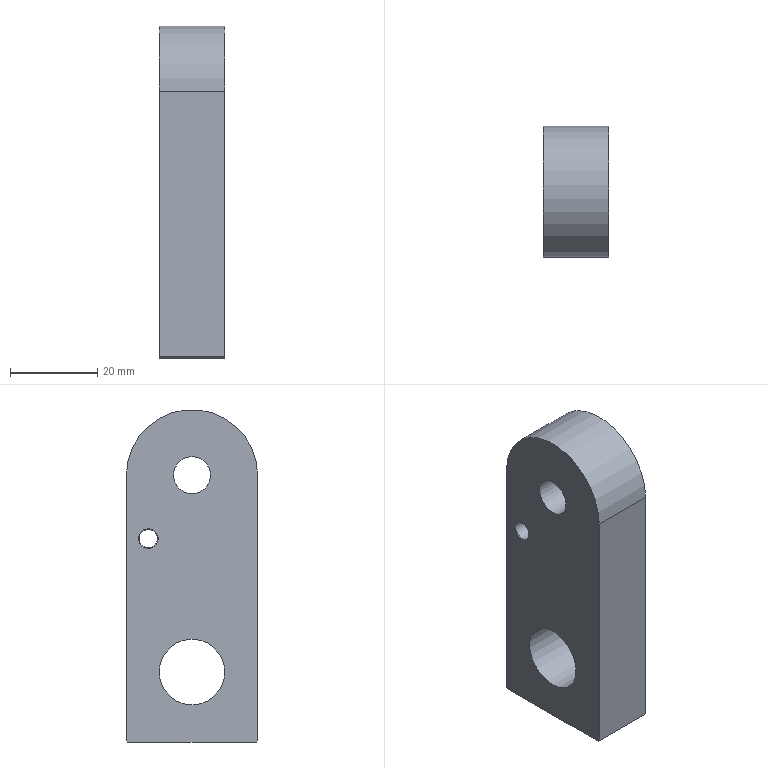Part | NX | 1 solid | 14 faces | box 15 x 30 x 76 mm | volume 28960 mm3 | plane 7 | cylinder 4 | cone 3 | commonest cylinder face diameters 4.2 x1 8.5 x1 15 x1 30 x1
STEP:
#1=CARTESIAN_POINT('',(0.,0.,0.3));
#2=VERTEX_POINT('',#1);
#3=CARTESIAN_POINT('',(0.,0.,61.));
#4=VERTEX_POINT('',#3);
#5=CARTESIAN_POINT('',(0.,0.,0.));
#6=DIRECTION('',(0.,0.,1.));
#7=VECTOR('',#6,1000.);
#8=LINE('',#5,#7);
#9=EDGE_CURVE('',#2,#4,#8,.T.);
#10=ORIENTED_EDGE('',*,*,#9,.F.);
#11=CARTESIAN_POINT('',(15.,0.,0.3));
#12=VERTEX_POINT('',#11);
#13=CARTESIAN_POINT('',(7.5,0.,0.3));
#14=DIRECTION('',(1.,0.,0.));
#15=VECTOR('',#14,1000.);
#16=LINE('',#13,#15);
#17=EDGE_CURVE('',#2,#12,#16,.T.);
#18=ORIENTED_EDGE('',*,*,#17,.T.);
#19=CARTESIAN_POINT('',(15.,0.,61.));
#20=VERTEX_POINT('',#19);
#21=CARTESIAN_POINT('',(15.,0.,0.));
#22=DIRECTION('',(0.,0.,1.));
#23=VECTOR('',#22,1000.);
#24=LINE('',#21,#23);
#25=EDGE_CURVE('',#12,#20,#24,.T.);
#26=ORIENTED_EDGE('',*,*,#25,.T.);
#27=CARTESIAN_POINT('',(7.5,0.,61.));
#28=DIRECTION('',(-1.,0.,0.));
#29=VECTOR('',#28,1000.);
#30=LINE('',#27,#29);
#31=EDGE_CURVE('',#20,#4,#30,.T.);
#32=ORIENTED_EDGE('',*,*,#31,.T.);
#33=EDGE_LOOP('',(#10,#18,#26,#32));
#34=FACE_BOUND('',#33,.T.);
#35=CARTESIAN_POINT('',(7.5,0.,0.));
#36=DIRECTION('',(0.,-1.,0.));
#37=DIRECTION('',(0.,0.,-1.));
#38=AXIS2_PLACEMENT_3D('',#35,#36,#37);
#39=PLANE('',#38);
#40=ADVANCED_FACE('',(#34),#39,.T.);
#41=CARTESIAN_POINT('',(0.,15.,23.5));
#42=VERTEX_POINT('',#41);
#43=CARTESIAN_POINT('',(0.,15.,16.));
#44=DIRECTION('',(-1.,0.,0.));
#45=DIRECTION('',(0.,0.,1.));
#46=AXIS2_PLACEMENT_3D('',#43,#44,#45);
#47=CIRCLE('',#46,7.5);
#48=EDGE_CURVE('',#42,#42,#47,.T.);
#49=ORIENTED_EDGE('',*,*,#48,.F.);
#50=EDGE_LOOP('',(#49));
#51=FACE_BOUND('',#50,.T.);
#52=CARTESIAN_POINT('',(0.,25.,48.75));
#53=VERTEX_POINT('',#52);
#54=CARTESIAN_POINT('',(0.,25.,46.5));
#55=DIRECTION('',(-1.,0.,0.));
#56=DIRECTION('',(0.,0.,1.));
#57=AXIS2_PLACEMENT_3D('',#54,#55,#56);
#58=CIRCLE('',#57,2.25);
#59=EDGE_CURVE('',#53,#53,#58,.F.);
#60=ORIENTED_EDGE('',*,*,#59,.T.);
#61=EDGE_LOOP('',(#60));
#62=FACE_BOUND('',#61,.T.);
#63=CARTESIAN_POINT('',(0.,15.,65.25));
#64=VERTEX_POINT('',#63);
#65=CARTESIAN_POINT('',(0.,15.,61.));
#66=DIRECTION('',(-1.,0.,0.));
#67=DIRECTION('',(0.,0.,1.));
#68=AXIS2_PLACEMENT_3D('',#65,#66,#67);
#69=CIRCLE('',#68,4.25);
#70=EDGE_CURVE('',#64,#64,#69,.T.);
#71=ORIENTED_EDGE('',*,*,#70,.F.);
#72=EDGE_LOOP('',(#71));
#73=FACE_BOUND('',#72,.T.);
#74=CARTESIAN_POINT('',(0.,30.,0.3));
#75=VERTEX_POINT('',#74);
#76=CARTESIAN_POINT('',(0.,30.,61.));
#77=VERTEX_POINT('',#76);
#78=CARTESIAN_POINT('',(0.,30.,0.));
#79=DIRECTION('',(0.,0.,1.));
#80=VECTOR('',#79,1000.);
#81=LINE('',#78,#80);
#82=EDGE_CURVE('',#75,#77,#81,.T.);
#83=ORIENTED_EDGE('',*,*,#82,.F.);
#84=CARTESIAN_POINT('',(0.,29.7,0.));
#85=VERTEX_POINT('',#84);
#86=CARTESIAN_POINT('',(0.,22.35,-7.35));
#87=DIRECTION('',(0.,0.7071,0.7071));
#88=VECTOR('',#87,1000.);
#89=LINE('',#86,#88);
#90=EDGE_CURVE('',#75,#85,#89,.F.);
#91=ORIENTED_EDGE('',*,*,#90,.T.);
#92=CARTESIAN_POINT('',(0.,0.3,0.));
#93=VERTEX_POINT('',#92);
#94=CARTESIAN_POINT('',(0.,15.,0.));
#95=DIRECTION('',(0.,-1.,0.));
#96=VECTOR('',#95,1000.);
#97=LINE('',#94,#96);
#98=EDGE_CURVE('',#85,#93,#97,.T.);
#99=ORIENTED_EDGE('',*,*,#98,.T.);
#100=CARTESIAN_POINT('',(0.,7.65,-7.35));
#101=DIRECTION('',(0.,0.7071,-0.7071));
#102=VECTOR('',#101,1000.);
#103=LINE('',#100,#102);
#104=EDGE_CURVE('',#93,#2,#103,.F.);
#105=ORIENTED_EDGE('',*,*,#104,.T.);
#106=ORIENTED_EDGE('',*,*,#9,.T.);
#107=CARTESIAN_POINT('',(0.,15.,61.));
#108=DIRECTION('',(-1.,0.,0.));
#109=DIRECTION('',(0.,0.,1.));
#110=AXIS2_PLACEMENT_3D('',#107,#108,#109);
#111=CIRCLE('',#110,15.);
#112=EDGE_CURVE('',#4,#77,#111,.T.);
#113=ORIENTED_EDGE('',*,*,#112,.T.);
#114=EDGE_LOOP('',(#83,#91,#99,#105,#106,#113));
#115=FACE_BOUND('',#114,.T.);
#116=CARTESIAN_POINT('',(0.,15.,0.));
#117=DIRECTION('',(-1.,0.,0.));
#118=DIRECTION('',(0.,0.,1.));
#119=AXIS2_PLACEMENT_3D('',#116,#117,#118);
#120=PLANE('',#119);
#121=ADVANCED_FACE('',(#51,#62,#73,#115),#120,.T.);
#122=CARTESIAN_POINT('',(15.,30.,0.3));
#123=VERTEX_POINT('',#122);
#124=CARTESIAN_POINT('',(15.,30.,61.));
#125=VERTEX_POINT('',#124);
#126=CARTESIAN_POINT('',(15.,30.,0.));
#127=DIRECTION('',(0.,0.,1.));
#128=VECTOR('',#127,1000.);
#129=LINE('',#126,#128);
#130=EDGE_CURVE('',#123,#125,#129,.T.);
#131=ORIENTED_EDGE('',*,*,#130,.F.);
#132=CARTESIAN_POINT('',(7.5,30.,0.3));
#133=DIRECTION('',(-1.,0.,0.));
#134=VECTOR('',#133,1000.);
#135=LINE('',#132,#134);
#136=EDGE_CURVE('',#123,#75,#135,.T.);
#137=ORIENTED_EDGE('',*,*,#136,.T.);
#138=ORIENTED_EDGE('',*,*,#82,.T.);
#139=CARTESIAN_POINT('',(7.5,30.,61.));
#140=DIRECTION('',(1.,0.,0.));
#141=VECTOR('',#140,1000.);
#142=LINE('',#139,#141);
#143=EDGE_CURVE('',#77,#125,#142,.T.);
#144=ORIENTED_EDGE('',*,*,#143,.T.);
#145=EDGE_LOOP('',(#131,#137,#138,#144));
#146=FACE_BOUND('',#145,.T.);
#147=CARTESIAN_POINT('',(7.5,30.,0.));
#148=DIRECTION('',(0.,1.,0.));
#149=DIRECTION('',(0.,0.,1.));
#150=AXIS2_PLACEMENT_3D('',#147,#148,#149);
#151=PLANE('',#150);
#152=ADVANCED_FACE('',(#146),#151,.T.);
#153=ORIENTED_EDGE('',*,*,#98,.F.);
#154=CARTESIAN_POINT('',(15.,29.7,0.));
#155=VERTEX_POINT('',#154);
#156=CARTESIAN_POINT('',(7.5,29.7,0.));
#157=DIRECTION('',(1.,0.,0.));
#158=VECTOR('',#157,1000.);
#159=LINE('',#156,#158);
#160=EDGE_CURVE('',#85,#155,#159,.T.);
#161=ORIENTED_EDGE('',*,*,#160,.T.);
#162=CARTESIAN_POINT('',(15.,0.3,0.));
#163=VERTEX_POINT('',#162);
#164=CARTESIAN_POINT('',(15.,15.,0.));
#165=DIRECTION('',(0.,1.,0.));
#166=VECTOR('',#165,1000.);
#167=LINE('',#164,#166);
#168=EDGE_CURVE('',#163,#155,#167,.T.);
#169=ORIENTED_EDGE('',*,*,#168,.F.);
#170=CARTESIAN_POINT('',(7.5,0.3,0.));
#171=DIRECTION('',(-1.,0.,0.));
#172=VECTOR('',#171,1000.);
#173=LINE('',#170,#172);
#174=EDGE_CURVE('',#163,#93,#173,.T.);
#175=ORIENTED_EDGE('',*,*,#174,.T.);
#176=EDGE_LOOP('',(#153,#161,#169,#175));
#177=FACE_BOUND('',#176,.T.);
#178=CARTESIAN_POINT('',(7.5,15.,0.));
#179=DIRECTION('',(0.,0.,-1.));
#180=DIRECTION('',(-1.,0.,0.));
#181=AXIS2_PLACEMENT_3D('',#178,#179,#180);
#182=PLANE('',#181);
#183=ADVANCED_FACE('',(#177),#182,.T.);
#184=CARTESIAN_POINT('',(15.,15.,23.5));
#185=VERTEX_POINT('',#184);
#186=CARTESIAN_POINT('',(15.,15.,16.));
#187=DIRECTION('',(-1.,0.,0.));
#188=DIRECTION('',(0.,0.,1.));
#189=AXIS2_PLACEMENT_3D('',#186,#187,#188);
#190=CIRCLE('',#189,7.5);
#191=EDGE_CURVE('',#185,#185,#190,.T.);
#192=ORIENTED_EDGE('',*,*,#191,.T.);
#193=EDGE_LOOP('',(#192));
#194=FACE_BOUND('',#193,.T.);
#195=CARTESIAN_POINT('',(15.,25.,44.25));
#196=VERTEX_POINT('',#195);
#197=CARTESIAN_POINT('',(15.,25.,46.5));
#198=DIRECTION('',(1.,0.,0.));
#199=DIRECTION('',(0.,0.,-1.));
#200=AXIS2_PLACEMENT_3D('',#197,#198,#199);
#201=CIRCLE('',#200,2.25);
#202=EDGE_CURVE('',#196,#196,#201,.F.);
#203=ORIENTED_EDGE('',*,*,#202,.T.);
#204=EDGE_LOOP('',(#203));
#205=FACE_BOUND('',#204,.T.);
#206=CARTESIAN_POINT('',(15.,15.,55.));
#207=VERTEX_POINT('',#206);
#208=CARTESIAN_POINT('',(15.,15.,61.));
#209=DIRECTION('',(1.,0.,0.));
#210=DIRECTION('',(0.,0.,-1.));
#211=AXIS2_PLACEMENT_3D('',#208,#209,#210);
#212=CIRCLE('',#211,6.);
#213=EDGE_CURVE('',#207,#207,#212,.F.);
#214=ORIENTED_EDGE('',*,*,#213,.T.);
#215=EDGE_LOOP('',(#214));
#216=FACE_BOUND('',#215,.T.);
#217=ORIENTED_EDGE('',*,*,#168,.T.);
#218=CARTESIAN_POINT('',(15.,22.35,-7.35));
#219=DIRECTION('',(0.,-0.7071,-0.7071));
#220=VECTOR('',#219,1000.);
#221=LINE('',#218,#220);
#222=EDGE_CURVE('',#155,#123,#221,.F.);
#223=ORIENTED_EDGE('',*,*,#222,.T.);
#224=ORIENTED_EDGE('',*,*,#130,.T.);
#225=CARTESIAN_POINT('',(15.,15.,61.));
#226=DIRECTION('',(1.,0.,0.));
#227=DIRECTION('',(0.,0.,-1.));
#228=AXIS2_PLACEMENT_3D('',#225,#226,#227);
#229=CIRCLE('',#228,15.);
#230=EDGE_CURVE('',#125,#20,#229,.T.);
#231=ORIENTED_EDGE('',*,*,#230,.T.);
#232=ORIENTED_EDGE('',*,*,#25,.F.);
#233=CARTESIAN_POINT('',(15.,7.65,-7.35));
#234=DIRECTION('',(0.,-0.7071,0.7071));
#235=VECTOR('',#234,1000.);
#236=LINE('',#233,#235);
#237=EDGE_CURVE('',#12,#163,#236,.F.);
#238=ORIENTED_EDGE('',*,*,#237,.T.);
#239=EDGE_LOOP('',(#217,#223,#224,#231,#232,#238));
#240=FACE_BOUND('',#239,.T.);
#241=CARTESIAN_POINT('',(15.,15.,0.));
#242=DIRECTION('',(1.,0.,0.));
#243=DIRECTION('',(0.,0.,-1.));
#244=AXIS2_PLACEMENT_3D('',#241,#242,#243);
#245=PLANE('',#244);
#246=ADVANCED_FACE('',(#194,#205,#216,#240),#245,.T.);
#247=ORIENTED_EDGE('',*,*,#230,.F.);
#248=ORIENTED_EDGE('',*,*,#143,.F.);
#249=ORIENTED_EDGE('',*,*,#112,.F.);
#250=ORIENTED_EDGE('',*,*,#31,.F.);
#251=EDGE_LOOP('',(#247,#248,#249,#250));
#252=FACE_BOUND('',#251,.T.);
#253=CARTESIAN_POINT('',(7.5,15.,61.));
#254=DIRECTION('',(-1.,0.,0.));
#255=DIRECTION('',(0.,0.,1.));
#256=AXIS2_PLACEMENT_3D('',#253,#254,#255);
#257=CYLINDRICAL_SURFACE('',#256,15.);
#258=ADVANCED_FACE('',(#252),#257,.T.);
#259=CARTESIAN_POINT('',(11.969,15.,56.75));
#260=VERTEX_POINT('',#259);
#261=CARTESIAN_POINT('',(11.969,15.,61.));
#262=DIRECTION('',(1.,0.,0.));
#263=DIRECTION('',(0.,0.,-1.));
#264=AXIS2_PLACEMENT_3D('',#261,#262,#263);
#265=CIRCLE('',#264,4.25);
#266=EDGE_CURVE('',#260,#260,#265,.T.);
#267=ORIENTED_EDGE('',*,*,#266,.T.);
#268=EDGE_LOOP('',(#267));
#269=FACE_BOUND('',#268,.T.);
#270=ORIENTED_EDGE('',*,*,#70,.T.);
#271=EDGE_LOOP('',(#270));
#272=FACE_BOUND('',#271,.T.);
#273=CARTESIAN_POINT('',(15.,15.,61.));
#274=DIRECTION('',(-1.,0.,0.));
#275=DIRECTION('',(0.,0.,1.));
#276=AXIS2_PLACEMENT_3D('',#273,#274,#275);
#277=CYLINDRICAL_SURFACE('',#276,4.25);
#278=ADVANCED_FACE('',(#269,#272),#277,.F.);
#279=ORIENTED_EDGE('',*,*,#266,.F.);
#280=EDGE_LOOP('',(#279));
#281=FACE_BOUND('',#280,.T.);
#282=ORIENTED_EDGE('',*,*,#213,.F.);
#283=EDGE_LOOP('',(#282));
#284=FACE_BOUND('',#283,.T.);
#285=CARTESIAN_POINT('',(15.,15.,61.));
#286=DIRECTION('',(1.,0.,0.));
#287=DIRECTION('',(0.,0.,-1.));
#288=AXIS2_PLACEMENT_3D('',#285,#286,#287);
#289=CONICAL_SURFACE('',#288,6.,0.5236);
#290=ADVANCED_FACE('',(#281,#284),#289,.F.);
#291=CARTESIAN_POINT('',(0.15,25.,48.6));
#292=VERTEX_POINT('',#291);
#293=CARTESIAN_POINT('',(0.15,25.,46.5));
#294=DIRECTION('',(-1.,0.,0.));
#295=DIRECTION('',(0.,0.,1.));
#296=AXIS2_PLACEMENT_3D('',#293,#294,#295);
#297=CIRCLE('',#296,2.1);
#298=EDGE_CURVE('',#292,#292,#297,.T.);
#299=ORIENTED_EDGE('',*,*,#298,.T.);
#300=EDGE_LOOP('',(#299));
#301=FACE_BOUND('',#300,.T.);
#302=CARTESIAN_POINT('',(14.85,25.,44.4));
#303=VERTEX_POINT('',#302);
#304=CARTESIAN_POINT('',(14.85,25.,46.5));
#305=DIRECTION('',(1.,0.,0.));
#306=DIRECTION('',(0.,0.,-1.));
#307=AXIS2_PLACEMENT_3D('',#304,#305,#306);
#308=CIRCLE('',#307,2.1);
#309=EDGE_CURVE('',#303,#303,#308,.T.);
#310=ORIENTED_EDGE('',*,*,#309,.T.);
#311=EDGE_LOOP('',(#310));
#312=FACE_BOUND('',#311,.T.);
#313=CARTESIAN_POINT('',(15.,25.,46.5));
#314=DIRECTION('',(-1.,0.,0.));
#315=DIRECTION('',(0.,0.,1.));
#316=AXIS2_PLACEMENT_3D('',#313,#314,#315);
#317=CYLINDRICAL_SURFACE('',#316,2.1);
#318=ADVANCED_FACE('',(#301,#312),#317,.F.);
#319=ORIENTED_EDGE('',*,*,#59,.F.);
#320=EDGE_LOOP('',(#319));
#321=FACE_BOUND('',#320,.T.);
#322=ORIENTED_EDGE('',*,*,#298,.F.);
#323=EDGE_LOOP('',(#322));
#324=FACE_BOUND('',#323,.T.);
#325=CARTESIAN_POINT('',(0.15,25.,46.5));
#326=DIRECTION('',(-1.,0.,0.));
#327=DIRECTION('',(0.,0.,1.));
#328=AXIS2_PLACEMENT_3D('',#325,#326,#327);
#329=CONICAL_SURFACE('',#328,2.1,0.7854);
#330=ADVANCED_FACE('',(#321,#324),#329,.F.);
#331=ORIENTED_EDGE('',*,*,#309,.F.);
#332=EDGE_LOOP('',(#331));
#333=FACE_BOUND('',#332,.T.);
#334=ORIENTED_EDGE('',*,*,#202,.F.);
#335=EDGE_LOOP('',(#334));
#336=FACE_BOUND('',#335,.T.);
#337=CARTESIAN_POINT('',(15.,25.,46.5));
#338=DIRECTION('',(1.,0.,0.));
#339=DIRECTION('',(0.,0.,-1.));
#340=AXIS2_PLACEMENT_3D('',#337,#338,#339);
#341=CONICAL_SURFACE('',#340,2.25,0.7854);
#342=ADVANCED_FACE('',(#333,#336),#341,.F.);
#343=ORIENTED_EDGE('',*,*,#48,.T.);
#344=EDGE_LOOP('',(#343));
#345=FACE_BOUND('',#344,.T.);
#346=ORIENTED_EDGE('',*,*,#191,.F.);
#347=EDGE_LOOP('',(#346));
#348=FACE_BOUND('',#347,.T.);
#349=CARTESIAN_POINT('',(15.,15.,16.));
#350=DIRECTION('',(-1.,0.,0.));
#351=DIRECTION('',(0.,0.,1.));
#352=AXIS2_PLACEMENT_3D('',#349,#350,#351);
#353=CYLINDRICAL_SURFACE('',#352,7.5);
#354=ADVANCED_FACE('',(#345,#348),#353,.F.);
#355=ORIENTED_EDGE('',*,*,#222,.F.);
#356=ORIENTED_EDGE('',*,*,#160,.F.);
#357=ORIENTED_EDGE('',*,*,#90,.F.);
#358=ORIENTED_EDGE('',*,*,#136,.F.);
#359=EDGE_LOOP('',(#355,#356,#357,#358));
#360=FACE_BOUND('',#359,.T.);
#361=CARTESIAN_POINT('',(7.5,30.,0.3));
#362=DIRECTION('',(0.,-0.7071,0.7071));
#363=DIRECTION('',(-1.,0.,0.));
#364=AXIS2_PLACEMENT_3D('',#361,#362,#363);
#365=PLANE('',#364);
#366=ADVANCED_FACE('',(#360),#365,.F.);
#367=ORIENTED_EDGE('',*,*,#104,.F.);
#368=ORIENTED_EDGE('',*,*,#174,.F.);
#369=ORIENTED_EDGE('',*,*,#237,.F.);
#370=ORIENTED_EDGE('',*,*,#17,.F.);
#371=EDGE_LOOP('',(#367,#368,#369,#370));
#372=FACE_BOUND('',#371,.T.);
#373=CARTESIAN_POINT('',(7.5,0.,0.3));
#374=DIRECTION('',(0.,0.7071,0.7071));
#375=DIRECTION('',(1.,0.,0.));
#376=AXIS2_PLACEMENT_3D('',#373,#374,#375);
#377=PLANE('',#376);
#378=ADVANCED_FACE('',(#372),#377,.F.);
#379=CLOSED_SHELL('',(#40,#121,#152,#183,#246,#258,#278,#290,#318,#330,#342,#354,#366,#378));
#380=MANIFOLD_SOLID_BREP('',#379);
#381=(LENGTH_UNIT()NAMED_UNIT(*)SI_UNIT(.MILLI.,.METRE.));
#382=UNCERTAINTY_MEASURE_WITH_UNIT(LENGTH_MEASURE(0.00001),#381,'','');
#383=(NAMED_UNIT(*)PLANE_ANGLE_UNIT()SI_UNIT($,.RADIAN.));
#384=(NAMED_UNIT(*)SI_UNIT($,.STERADIAN.)SOLID_ANGLE_UNIT());
#385=(GEOMETRIC_REPRESENTATION_CONTEXT(3)GLOBAL_UNCERTAINTY_ASSIGNED_CONTEXT((#382))GLOBAL_UNIT_ASSIGNED_CONTEXT((#381,#383,#384))REPRESENTATION_CONTEXT('',''));
#386=ADVANCED_BREP_SHAPE_REPRESENTATION('',(#380),#385);